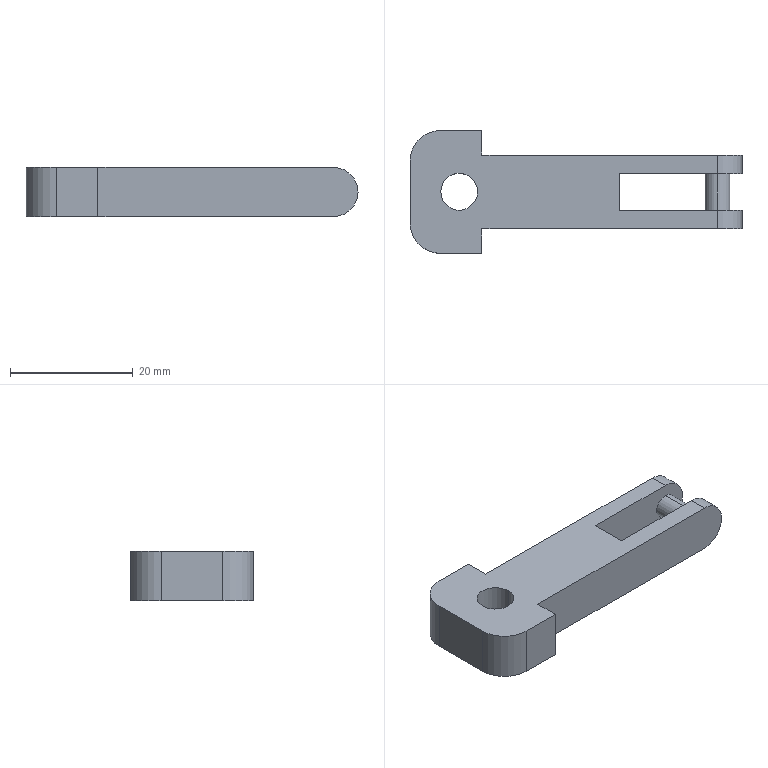Part | SolidWorks | features Fillet 2, ICE 2, Extrusion 1 | 1 solid | 22 faces | box 54 x 20 x 8 mm | volume 4696 mm3 | plane 12 | cylinder 10 | commonest cylinder face diameters 8 x4 4 x2 6 x2 10 x2
STEP:
#1=CARTESIAN_POINT('',(-27.268,0.,0.));
#2=VERTEX_POINT('',#1);
#3=CARTESIAN_POINT('',(-21.268,0.,0.));
#4=VERTEX_POINT('',#3);
#5=CARTESIAN_POINT('',(-24.268,0.,0.));
#6=DIRECTION('',(0.,0.,1.));
#7=DIRECTION('',(1.,0.,0.));
#8=AXIS2_PLACEMENT_3D('',#5,#6,#7);
#9=CIRCLE('',#8,3.);
#10=EDGE_CURVE('',#2,#4,#9,.T.);
#11=ORIENTED_EDGE('',*,*,#10,.F.);
#12=CARTESIAN_POINT('',(-27.268,0.,8.));
#13=VERTEX_POINT('',#12);
#14=CARTESIAN_POINT('',(-27.268,0.,0.));
#15=DIRECTION('',(0.,0.,1.));
#16=VECTOR('',#15,1000.);
#17=LINE('',#14,#16);
#18=EDGE_CURVE('',#2,#13,#17,.T.);
#19=ORIENTED_EDGE('',*,*,#18,.T.);
#20=CARTESIAN_POINT('',(-21.268,0.,8.));
#21=VERTEX_POINT('',#20);
#22=CARTESIAN_POINT('',(-24.268,0.,8.));
#23=DIRECTION('',(0.,0.,1.));
#24=DIRECTION('',(1.,0.,0.));
#25=AXIS2_PLACEMENT_3D('',#22,#23,#24);
#26=CIRCLE('',#25,3.);
#27=EDGE_CURVE('',#13,#21,#26,.T.);
#28=ORIENTED_EDGE('',*,*,#27,.T.);
#29=CARTESIAN_POINT('',(-21.268,0.,0.));
#30=DIRECTION('',(0.,0.,1.));
#31=VECTOR('',#30,1000.);
#32=LINE('',#29,#31);
#33=EDGE_CURVE('',#4,#21,#32,.T.);
#34=ORIENTED_EDGE('',*,*,#33,.F.);
#35=EDGE_LOOP('',(#11,#19,#28,#34));
#36=FACE_OUTER_BOUND('',#35,.T.);
#37=CARTESIAN_POINT('',(-24.268,0.,0.));
#38=DIRECTION('',(0.,0.,1.));
#39=DIRECTION('',(1.,0.,0.));
#40=AXIS2_PLACEMENT_3D('',#37,#38,#39);
#41=CYLINDRICAL_SURFACE('',#40,3.);
#42=ADVANCED_FACE('',(#36),#41,.F.);
#43=CARTESIAN_POINT('',(17.732,2.96,6.));
#44=VERTEX_POINT('',#43);
#45=CARTESIAN_POINT('',(17.732,2.96,2.));
#46=VERTEX_POINT('',#45);
#47=CARTESIAN_POINT('',(17.732,2.96,4.));
#48=DIRECTION('',(0.,1.,0.));
#49=DIRECTION('',(-1.,0.,0.));
#50=AXIS2_PLACEMENT_3D('',#47,#48,#49);
#51=CIRCLE('',#50,2.);
#52=EDGE_CURVE('',#44,#46,#51,.T.);
#53=ORIENTED_EDGE('',*,*,#52,.F.);
#54=CARTESIAN_POINT('',(17.732,-3.04,6.));
#55=VERTEX_POINT('',#54);
#56=CARTESIAN_POINT('',(17.732,5.96,6.));
#57=DIRECTION('',(0.,-1.,0.));
#58=VECTOR('',#57,1000.);
#59=LINE('',#56,#58);
#60=EDGE_CURVE('',#44,#55,#59,.T.);
#61=ORIENTED_EDGE('',*,*,#60,.T.);
#62=CARTESIAN_POINT('',(17.732,-3.04,2.));
#63=VERTEX_POINT('',#62);
#64=CARTESIAN_POINT('',(17.732,-3.04,4.));
#65=DIRECTION('',(0.,-1.,0.));
#66=DIRECTION('',(0.,0.,-1.));
#67=AXIS2_PLACEMENT_3D('',#64,#65,#66);
#68=CIRCLE('',#67,2.);
#69=EDGE_CURVE('',#63,#55,#68,.T.);
#70=ORIENTED_EDGE('',*,*,#69,.F.);
#71=CARTESIAN_POINT('',(17.732,5.96,2.));
#72=DIRECTION('',(0.,-1.,0.));
#73=VECTOR('',#72,1000.);
#74=LINE('',#71,#73);
#75=EDGE_CURVE('',#46,#63,#74,.T.);
#76=ORIENTED_EDGE('',*,*,#75,.F.);
#77=EDGE_LOOP('',(#53,#61,#70,#76));
#78=FACE_OUTER_BOUND('',#77,.T.);
#79=CARTESIAN_POINT('',(17.732,5.96,4.));
#80=DIRECTION('',(0.,-1.,0.));
#81=DIRECTION('',(0.,0.,-1.));
#82=AXIS2_PLACEMENT_3D('',#79,#80,#81);
#83=CYLINDRICAL_SURFACE('',#82,2.);
#84=ADVANCED_FACE('',(#78),#83,.T.);
#85=CARTESIAN_POINT('',(17.732,5.96,8.));
#86=VERTEX_POINT('',#85);
#87=CARTESIAN_POINT('',(21.732,5.96,4.));
#88=VERTEX_POINT('',#87);
#89=CARTESIAN_POINT('',(17.732,5.96,4.));
#90=DIRECTION('',(0.,1.,0.));
#91=DIRECTION('',(0.,0.,-1.));
#92=AXIS2_PLACEMENT_3D('',#89,#90,#91);
#93=CIRCLE('',#92,4.);
#94=EDGE_CURVE('',#86,#88,#93,.T.);
#95=ORIENTED_EDGE('',*,*,#94,.T.);
#96=CARTESIAN_POINT('',(17.732,5.96,0.));
#97=VERTEX_POINT('',#96);
#98=CARTESIAN_POINT('',(17.732,5.96,4.));
#99=DIRECTION('',(0.,1.,0.));
#100=DIRECTION('',(0.,0.,-1.));
#101=AXIS2_PLACEMENT_3D('',#98,#99,#100);
#102=CIRCLE('',#101,4.);
#103=EDGE_CURVE('',#88,#97,#102,.T.);
#104=ORIENTED_EDGE('',*,*,#103,.T.);
#105=CARTESIAN_POINT('',(-20.559,5.96,0.));
#106=VERTEX_POINT('',#105);
#107=CARTESIAN_POINT('',(-20.559,5.96,0.));
#108=DIRECTION('',(-1.,0.,0.));
#109=VECTOR('',#108,1000.);
#110=LINE('',#107,#109);
#111=EDGE_CURVE('',#97,#106,#110,.T.);
#112=ORIENTED_EDGE('',*,*,#111,.T.);
#113=CARTESIAN_POINT('',(-20.559,5.96,8.));
#114=VERTEX_POINT('',#113);
#115=CARTESIAN_POINT('',(-20.559,5.96,8.));
#116=DIRECTION('',(0.,0.,-1.));
#117=VECTOR('',#116,1000.);
#118=LINE('',#115,#117);
#119=EDGE_CURVE('',#114,#106,#118,.T.);
#120=ORIENTED_EDGE('',*,*,#119,.F.);
#121=CARTESIAN_POINT('',(-20.559,5.96,8.));
#122=DIRECTION('',(-1.,0.,0.));
#123=VECTOR('',#122,1000.);
#124=LINE('',#121,#123);
#125=EDGE_CURVE('',#86,#114,#124,.T.);
#126=ORIENTED_EDGE('',*,*,#125,.F.);
#127=EDGE_LOOP('',(#95,#104,#112,#120,#126));
#128=FACE_OUTER_BOUND('',#127,.T.);
#129=CARTESIAN_POINT('',(-20.559,5.96,8.));
#130=DIRECTION('',(0.,-1.,0.));
#131=DIRECTION('',(0.,0.,-1.));
#132=AXIS2_PLACEMENT_3D('',#129,#130,#131);
#133=PLANE('',#132);
#134=ADVANCED_FACE('',(#128),#133,.F.);
#135=CARTESIAN_POINT('',(-20.559,9.96,0.));
#136=VERTEX_POINT('',#135);
#137=CARTESIAN_POINT('',(-20.559,9.96,0.));
#138=DIRECTION('',(0.,1.,0.));
#139=VECTOR('',#138,1000.);
#140=LINE('',#137,#139);
#141=EDGE_CURVE('',#106,#136,#140,.T.);
#142=ORIENTED_EDGE('',*,*,#141,.T.);
#143=CARTESIAN_POINT('',(-20.559,9.96,8.));
#144=VERTEX_POINT('',#143);
#145=CARTESIAN_POINT('',(-20.559,9.96,8.));
#146=DIRECTION('',(0.,0.,-1.));
#147=VECTOR('',#146,1000.);
#148=LINE('',#145,#147);
#149=EDGE_CURVE('',#144,#136,#148,.T.);
#150=ORIENTED_EDGE('',*,*,#149,.F.);
#151=CARTESIAN_POINT('',(-20.559,9.96,8.));
#152=DIRECTION('',(0.,1.,0.));
#153=VECTOR('',#152,1000.);
#154=LINE('',#151,#153);
#155=EDGE_CURVE('',#114,#144,#154,.T.);
#156=ORIENTED_EDGE('',*,*,#155,.F.);
#157=ORIENTED_EDGE('',*,*,#119,.T.);
#158=EDGE_LOOP('',(#142,#150,#156,#157));
#159=FACE_OUTER_BOUND('',#158,.T.);
#160=CARTESIAN_POINT('',(-20.559,9.96,8.));
#161=DIRECTION('',(-1.,0.,0.));
#162=DIRECTION('',(0.,0.,1.));
#163=AXIS2_PLACEMENT_3D('',#160,#161,#162);
#164=PLANE('',#163);
#165=ADVANCED_FACE('',(#159),#164,.F.);
#166=CARTESIAN_POINT('',(-27.268,9.96,0.));
#167=VERTEX_POINT('',#166);
#168=CARTESIAN_POINT('',(-20.559,9.96,0.));
#169=DIRECTION('',(-1.,0.,0.));
#170=VECTOR('',#169,1000.);
#171=LINE('',#168,#170);
#172=EDGE_CURVE('',#136,#167,#171,.T.);
#173=ORIENTED_EDGE('',*,*,#172,.T.);
#174=CARTESIAN_POINT('',(-27.268,9.96,8.));
#175=VERTEX_POINT('',#174);
#176=CARTESIAN_POINT('',(-27.268,9.96,8.));
#177=DIRECTION('',(0.,0.,1.));
#178=VECTOR('',#177,1000.);
#179=LINE('',#176,#178);
#180=EDGE_CURVE('',#167,#175,#179,.T.);
#181=ORIENTED_EDGE('',*,*,#180,.T.);
#182=CARTESIAN_POINT('',(-20.559,9.96,8.));
#183=DIRECTION('',(-1.,0.,0.));
#184=VECTOR('',#183,1000.);
#185=LINE('',#182,#184);
#186=EDGE_CURVE('',#144,#175,#185,.T.);
#187=ORIENTED_EDGE('',*,*,#186,.F.);
#188=ORIENTED_EDGE('',*,*,#149,.T.);
#189=EDGE_LOOP('',(#173,#181,#187,#188));
#190=FACE_OUTER_BOUND('',#189,.T.);
#191=CARTESIAN_POINT('',(-20.559,9.96,8.));
#192=DIRECTION('',(0.,-1.,0.));
#193=DIRECTION('',(0.,0.,-1.));
#194=AXIS2_PLACEMENT_3D('',#191,#192,#193);
#195=PLANE('',#194);
#196=ADVANCED_FACE('',(#190),#195,.F.);
#197=CARTESIAN_POINT('',(-32.268,4.96,0.));
#198=VERTEX_POINT('',#197);
#199=CARTESIAN_POINT('',(-32.268,-5.04,0.));
#200=VERTEX_POINT('',#199);
#201=CARTESIAN_POINT('',(-32.268,-10.04,0.));
#202=DIRECTION('',(0.,-1.,0.));
#203=VECTOR('',#202,1000.);
#204=LINE('',#201,#203);
#205=EDGE_CURVE('',#198,#200,#204,.T.);
#206=ORIENTED_EDGE('',*,*,#205,.T.);
#207=CARTESIAN_POINT('',(-32.268,-5.04,8.));
#208=VERTEX_POINT('',#207);
#209=CARTESIAN_POINT('',(-32.268,-5.04,8.));
#210=DIRECTION('',(0.,0.,1.));
#211=VECTOR('',#210,1000.);
#212=LINE('',#209,#211);
#213=EDGE_CURVE('',#200,#208,#212,.T.);
#214=ORIENTED_EDGE('',*,*,#213,.T.);
#215=CARTESIAN_POINT('',(-32.268,4.96,8.));
#216=VERTEX_POINT('',#215);
#217=CARTESIAN_POINT('',(-32.268,9.96,8.));
#218=DIRECTION('',(0.,-1.,0.));
#219=VECTOR('',#218,1000.);
#220=LINE('',#217,#219);
#221=EDGE_CURVE('',#216,#208,#220,.T.);
#222=ORIENTED_EDGE('',*,*,#221,.F.);
#223=CARTESIAN_POINT('',(-32.268,4.96,8.));
#224=DIRECTION('',(0.,0.,-1.));
#225=VECTOR('',#224,1000.);
#226=LINE('',#223,#225);
#227=EDGE_CURVE('',#216,#198,#226,.T.);
#228=ORIENTED_EDGE('',*,*,#227,.T.);
#229=EDGE_LOOP('',(#206,#214,#222,#228));
#230=FACE_OUTER_BOUND('',#229,.T.);
#231=CARTESIAN_POINT('',(-32.268,-10.04,8.));
#232=DIRECTION('',(1.,0.,0.));
#233=DIRECTION('',(0.,0.,-1.));
#234=AXIS2_PLACEMENT_3D('',#231,#232,#233);
#235=PLANE('',#234);
#236=ADVANCED_FACE('',(#230),#235,.F.);
#237=CARTESIAN_POINT('',(-27.268,-10.04,8.));
#238=VERTEX_POINT('',#237);
#239=CARTESIAN_POINT('',(-20.559,-10.04,8.));
#240=VERTEX_POINT('',#239);
#241=CARTESIAN_POINT('',(-32.268,-10.04,8.));
#242=DIRECTION('',(1.,0.,0.));
#243=VECTOR('',#242,1000.);
#244=LINE('',#241,#243);
#245=EDGE_CURVE('',#238,#240,#244,.T.);
#246=ORIENTED_EDGE('',*,*,#245,.F.);
#247=CARTESIAN_POINT('',(-27.268,-10.04,0.));
#248=VERTEX_POINT('',#247);
#249=CARTESIAN_POINT('',(-27.268,-10.04,8.));
#250=DIRECTION('',(0.,0.,-1.));
#251=VECTOR('',#250,1000.);
#252=LINE('',#249,#251);
#253=EDGE_CURVE('',#238,#248,#252,.T.);
#254=ORIENTED_EDGE('',*,*,#253,.T.);
#255=CARTESIAN_POINT('',(-20.559,-10.04,0.));
#256=VERTEX_POINT('',#255);
#257=CARTESIAN_POINT('',(-32.268,-10.04,0.));
#258=DIRECTION('',(1.,0.,0.));
#259=VECTOR('',#258,1000.);
#260=LINE('',#257,#259);
#261=EDGE_CURVE('',#248,#256,#260,.T.);
#262=ORIENTED_EDGE('',*,*,#261,.T.);
#263=CARTESIAN_POINT('',(-20.559,-10.04,8.));
#264=DIRECTION('',(0.,0.,-1.));
#265=VECTOR('',#264,1000.);
#266=LINE('',#263,#265);
#267=EDGE_CURVE('',#240,#256,#266,.T.);
#268=ORIENTED_EDGE('',*,*,#267,.F.);
#269=EDGE_LOOP('',(#246,#254,#262,#268));
#270=FACE_OUTER_BOUND('',#269,.T.);
#271=CARTESIAN_POINT('',(-32.268,-10.04,8.));
#272=DIRECTION('',(0.,1.,0.));
#273=DIRECTION('',(0.,0.,1.));
#274=AXIS2_PLACEMENT_3D('',#271,#272,#273);
#275=PLANE('',#274);
#276=ADVANCED_FACE('',(#270),#275,.F.);
#277=CARTESIAN_POINT('',(-20.559,-6.04,0.));
#278=VERTEX_POINT('',#277);
#279=CARTESIAN_POINT('',(-20.559,-6.04,0.));
#280=DIRECTION('',(0.,1.,0.));
#281=VECTOR('',#280,1000.);
#282=LINE('',#279,#281);
#283=EDGE_CURVE('',#256,#278,#282,.T.);
#284=ORIENTED_EDGE('',*,*,#283,.T.);
#285=CARTESIAN_POINT('',(-20.559,-6.04,8.));
#286=VERTEX_POINT('',#285);
#287=CARTESIAN_POINT('',(-20.559,-6.04,8.));
#288=DIRECTION('',(0.,0.,-1.));
#289=VECTOR('',#288,1000.);
#290=LINE('',#287,#289);
#291=EDGE_CURVE('',#286,#278,#290,.T.);
#292=ORIENTED_EDGE('',*,*,#291,.F.);
#293=CARTESIAN_POINT('',(-20.559,-6.04,8.));
#294=DIRECTION('',(0.,1.,0.));
#295=VECTOR('',#294,1000.);
#296=LINE('',#293,#295);
#297=EDGE_CURVE('',#240,#286,#296,.T.);
#298=ORIENTED_EDGE('',*,*,#297,.F.);
#299=ORIENTED_EDGE('',*,*,#267,.T.);
#300=EDGE_LOOP('',(#284,#292,#298,#299));
#301=FACE_OUTER_BOUND('',#300,.T.);
#302=CARTESIAN_POINT('',(-20.559,-6.04,8.));
#303=DIRECTION('',(-1.,0.,0.));
#304=DIRECTION('',(0.,0.,1.));
#305=AXIS2_PLACEMENT_3D('',#302,#303,#304);
#306=PLANE('',#305);
#307=ADVANCED_FACE('',(#301),#306,.F.);
#308=CARTESIAN_POINT('',(17.732,-6.04,0.));
#309=VERTEX_POINT('',#308);
#310=CARTESIAN_POINT('',(-20.559,-6.04,0.));
#311=DIRECTION('',(1.,0.,0.));
#312=VECTOR('',#311,1000.);
#313=LINE('',#310,#312);
#314=EDGE_CURVE('',#278,#309,#313,.T.);
#315=ORIENTED_EDGE('',*,*,#314,.T.);
#316=CARTESIAN_POINT('',(21.732,-6.04,4.));
#317=VERTEX_POINT('',#316);
#318=CARTESIAN_POINT('',(17.732,-6.04,4.));
#319=DIRECTION('',(0.,-1.,0.));
#320=DIRECTION('',(0.,0.,1.));
#321=AXIS2_PLACEMENT_3D('',#318,#319,#320);
#322=CIRCLE('',#321,4.);
#323=EDGE_CURVE('',#309,#317,#322,.T.);
#324=ORIENTED_EDGE('',*,*,#323,.T.);
#325=CARTESIAN_POINT('',(17.732,-6.04,8.));
#326=VERTEX_POINT('',#325);
#327=CARTESIAN_POINT('',(17.732,-6.04,4.));
#328=DIRECTION('',(0.,-1.,0.));
#329=DIRECTION('',(0.,0.,1.));
#330=AXIS2_PLACEMENT_3D('',#327,#328,#329);
#331=CIRCLE('',#330,4.);
#332=EDGE_CURVE('',#317,#326,#331,.T.);
#333=ORIENTED_EDGE('',*,*,#332,.T.);
#334=CARTESIAN_POINT('',(-20.559,-6.04,8.));
#335=DIRECTION('',(1.,0.,0.));
#336=VECTOR('',#335,1000.);
#337=LINE('',#334,#336);
#338=EDGE_CURVE('',#286,#326,#337,.T.);
#339=ORIENTED_EDGE('',*,*,#338,.F.);
#340=ORIENTED_EDGE('',*,*,#291,.T.);
#341=EDGE_LOOP('',(#315,#324,#333,#339,#340));
#342=FACE_OUTER_BOUND('',#341,.T.);
#343=CARTESIAN_POINT('',(-20.559,-6.04,8.));
#344=DIRECTION('',(0.,1.,0.));
#345=DIRECTION('',(0.,0.,1.));
#346=AXIS2_PLACEMENT_3D('',#343,#344,#345);
#347=PLANE('',#346);
#348=ADVANCED_FACE('',(#342),#347,.F.);
#349=ORIENTED_EDGE('',*,*,#69,.T.);
#350=CARTESIAN_POINT('',(17.732,-3.04,4.));
#351=DIRECTION('',(0.,-1.,0.));
#352=DIRECTION('',(0.,0.,-1.));
#353=AXIS2_PLACEMENT_3D('',#350,#351,#352);
#354=CIRCLE('',#353,2.);
#355=EDGE_CURVE('',#55,#63,#354,.T.);
#356=ORIENTED_EDGE('',*,*,#355,.T.);
#357=EDGE_LOOP('',(#349,#356));
#358=FACE_BOUND('',#357,.T.);
#359=CARTESIAN_POINT('',(17.732,-3.04,8.));
#360=VERTEX_POINT('',#359);
#361=CARTESIAN_POINT('',(21.732,-3.04,4.));
#362=VERTEX_POINT('',#361);
#363=CARTESIAN_POINT('',(17.732,-3.04,4.));
#364=DIRECTION('',(0.,1.,0.));
#365=DIRECTION('',(0.,0.,-1.));
#366=AXIS2_PLACEMENT_3D('',#363,#364,#365);
#367=CIRCLE('',#366,4.);
#368=EDGE_CURVE('',#360,#362,#367,.T.);
#369=ORIENTED_EDGE('',*,*,#368,.T.);
#370=CARTESIAN_POINT('',(17.732,-3.04,0.));
#371=VERTEX_POINT('',#370);
#372=CARTESIAN_POINT('',(17.732,-3.04,4.));
#373=DIRECTION('',(0.,1.,0.));
#374=DIRECTION('',(0.,0.,-1.));
#375=AXIS2_PLACEMENT_3D('',#372,#373,#374);
#376=CIRCLE('',#375,4.);
#377=EDGE_CURVE('',#362,#371,#376,.T.);
#378=ORIENTED_EDGE('',*,*,#377,.T.);
#379=CARTESIAN_POINT('',(1.732,-3.04,0.));
#380=VERTEX_POINT('',#379);
#381=CARTESIAN_POINT('',(1.732,-3.04,0.));
#382=DIRECTION('',(-1.,0.,0.));
#383=VECTOR('',#382,1000.);
#384=LINE('',#381,#383);
#385=EDGE_CURVE('',#371,#380,#384,.T.);
#386=ORIENTED_EDGE('',*,*,#385,.T.);
#387=CARTESIAN_POINT('',(1.732,-3.04,8.));
#388=VERTEX_POINT('',#387);
#389=CARTESIAN_POINT('',(1.732,-3.04,8.));
#390=DIRECTION('',(0.,0.,-1.));
#391=VECTOR('',#390,1000.);
#392=LINE('',#389,#391);
#393=EDGE_CURVE('',#388,#380,#392,.T.);
#394=ORIENTED_EDGE('',*,*,#393,.F.);
#395=CARTESIAN_POINT('',(1.732,-3.04,8.));
#396=DIRECTION('',(-1.,0.,0.));
#397=VECTOR('',#396,1000.);
#398=LINE('',#395,#397);
#399=EDGE_CURVE('',#360,#388,#398,.T.);
#400=ORIENTED_EDGE('',*,*,#399,.F.);
#401=EDGE_LOOP('',(#369,#378,#386,#394,#400));
#402=FACE_OUTER_BOUND('',#401,.T.);
#403=CARTESIAN_POINT('',(1.732,-3.04,8.));
#404=DIRECTION('',(0.,-1.,0.));
#405=DIRECTION('',(0.,0.,-1.));
#406=AXIS2_PLACEMENT_3D('',#403,#404,#405);
#407=PLANE('',#406);
#408=ADVANCED_FACE('',(#358,#402),#407,.F.);
#409=CARTESIAN_POINT('',(1.732,2.96,0.));
#410=VERTEX_POINT('',#409);
#411=CARTESIAN_POINT('',(1.732,2.96,0.));
#412=DIRECTION('',(0.,1.,0.));
#413=VECTOR('',#412,1000.);
#414=LINE('',#411,#413);
#415=EDGE_CURVE('',#380,#410,#414,.T.);
#416=ORIENTED_EDGE('',*,*,#415,.T.);
#417=CARTESIAN_POINT('',(1.732,2.96,8.));
#418=VERTEX_POINT('',#417);
#419=CARTESIAN_POINT('',(1.732,2.96,8.));
#420=DIRECTION('',(0.,0.,-1.));
#421=VECTOR('',#420,1000.);
#422=LINE('',#419,#421);
#423=EDGE_CURVE('',#418,#410,#422,.T.);
#424=ORIENTED_EDGE('',*,*,#423,.F.);
#425=CARTESIAN_POINT('',(1.732,2.96,8.));
#426=DIRECTION('',(0.,1.,0.));
#427=VECTOR('',#426,1000.);
#428=LINE('',#425,#427);
#429=EDGE_CURVE('',#388,#418,#428,.T.);
#430=ORIENTED_EDGE('',*,*,#429,.F.);
#431=ORIENTED_EDGE('',*,*,#393,.T.);
#432=EDGE_LOOP('',(#416,#424,#430,#431));
#433=FACE_OUTER_BOUND('',#432,.T.);
#434=CARTESIAN_POINT('',(1.732,2.96,8.));
#435=DIRECTION('',(-1.,0.,0.));
#436=DIRECTION('',(0.,0.,1.));
#437=AXIS2_PLACEMENT_3D('',#434,#435,#436);
#438=PLANE('',#437);
#439=ADVANCED_FACE('',(#433),#438,.F.);
#440=CARTESIAN_POINT('',(17.732,2.96,4.));
#441=DIRECTION('',(0.,1.,0.));
#442=DIRECTION('',(-1.,0.,0.));
#443=AXIS2_PLACEMENT_3D('',#440,#441,#442);
#444=CIRCLE('',#443,2.);
#445=EDGE_CURVE('',#46,#44,#444,.T.);
#446=ORIENTED_EDGE('',*,*,#445,.T.);
#447=ORIENTED_EDGE('',*,*,#52,.T.);
#448=EDGE_LOOP('',(#446,#447));
#449=FACE_BOUND('',#448,.T.);
#450=CARTESIAN_POINT('',(17.732,2.96,0.));
#451=VERTEX_POINT('',#450);
#452=CARTESIAN_POINT('',(1.732,2.96,0.));
#453=DIRECTION('',(1.,0.,0.));
#454=VECTOR('',#453,1000.);
#455=LINE('',#452,#454);
#456=EDGE_CURVE('',#410,#451,#455,.T.);
#457=ORIENTED_EDGE('',*,*,#456,.T.);
#458=CARTESIAN_POINT('',(21.732,2.96,4.));
#459=VERTEX_POINT('',#458);
#460=CARTESIAN_POINT('',(17.732,2.96,4.));
#461=DIRECTION('',(0.,-1.,0.));
#462=DIRECTION('',(-1.,0.,0.));
#463=AXIS2_PLACEMENT_3D('',#460,#461,#462);
#464=CIRCLE('',#463,4.);
#465=EDGE_CURVE('',#451,#459,#464,.T.);
#466=ORIENTED_EDGE('',*,*,#465,.T.);
#467=CARTESIAN_POINT('',(17.732,2.96,8.));
#468=VERTEX_POINT('',#467);
#469=CARTESIAN_POINT('',(17.732,2.96,4.));
#470=DIRECTION('',(0.,-1.,0.));
#471=DIRECTION('',(-1.,0.,0.));
#472=AXIS2_PLACEMENT_3D('',#469,#470,#471);
#473=CIRCLE('',#472,4.);
#474=EDGE_CURVE('',#459,#468,#473,.T.);
#475=ORIENTED_EDGE('',*,*,#474,.T.);
#476=CARTESIAN_POINT('',(1.732,2.96,8.));
#477=DIRECTION('',(1.,0.,0.));
#478=VECTOR('',#477,1000.);
#479=LINE('',#476,#478);
#480=EDGE_CURVE('',#418,#468,#479,.T.);
#481=ORIENTED_EDGE('',*,*,#480,.F.);
#482=ORIENTED_EDGE('',*,*,#423,.T.);
#483=EDGE_LOOP('',(#457,#466,#475,#481,#482));
#484=FACE_OUTER_BOUND('',#483,.T.);
#485=CARTESIAN_POINT('',(1.732,2.96,8.));
#486=DIRECTION('',(0.,1.,0.));
#487=DIRECTION('',(-1.,0.,0.));
#488=AXIS2_PLACEMENT_3D('',#485,#486,#487);
#489=PLANE('',#488);
#490=ADVANCED_FACE('',(#449,#484),#489,.F.);
#491=CARTESIAN_POINT('',(-24.268,0.,8.));
#492=DIRECTION('',(0.,0.,1.));
#493=DIRECTION('',(1.,0.,0.));
#494=AXIS2_PLACEMENT_3D('',#491,#492,#493);
#495=CIRCLE('',#494,3.);
#496=EDGE_CURVE('',#21,#13,#495,.T.);
#497=ORIENTED_EDGE('',*,*,#496,.F.);
#498=ORIENTED_EDGE('',*,*,#27,.F.);
#499=EDGE_LOOP('',(#497,#498));
#500=FACE_BOUND('',#499,.T.);
#501=ORIENTED_EDGE('',*,*,#338,.T.);
#502=CARTESIAN_POINT('',(17.732,0.,8.));
#503=DIRECTION('',(0.,1.,0.));
#504=VECTOR('',#503,1000.);
#505=LINE('',#502,#504);
#506=EDGE_CURVE('',#326,#360,#505,.T.);
#507=ORIENTED_EDGE('',*,*,#506,.T.);
#508=ORIENTED_EDGE('',*,*,#399,.T.);
#509=ORIENTED_EDGE('',*,*,#429,.T.);
#510=ORIENTED_EDGE('',*,*,#480,.T.);
#511=CARTESIAN_POINT('',(17.732,0.,8.));
#512=DIRECTION('',(0.,1.,0.));
#513=VECTOR('',#512,1000.);
#514=LINE('',#511,#513);
#515=EDGE_CURVE('',#468,#86,#514,.T.);
#516=ORIENTED_EDGE('',*,*,#515,.T.);
#517=ORIENTED_EDGE('',*,*,#125,.T.);
#518=ORIENTED_EDGE('',*,*,#155,.T.);
#519=ORIENTED_EDGE('',*,*,#186,.T.);
#520=CARTESIAN_POINT('',(-27.268,4.96,8.));
#521=DIRECTION('',(0.,0.,1.));
#522=DIRECTION('',(-1.,0.,0.));
#523=AXIS2_PLACEMENT_3D('',#520,#521,#522);
#524=CIRCLE('',#523,5.);
#525=EDGE_CURVE('',#175,#216,#524,.T.);
#526=ORIENTED_EDGE('',*,*,#525,.T.);
#527=ORIENTED_EDGE('',*,*,#221,.T.);
#528=CARTESIAN_POINT('',(-27.268,-5.04,8.));
#529=DIRECTION('',(0.,0.,1.));
#530=DIRECTION('',(-1.,0.,0.));
#531=AXIS2_PLACEMENT_3D('',#528,#529,#530);
#532=CIRCLE('',#531,5.);
#533=EDGE_CURVE('',#208,#238,#532,.T.);
#534=ORIENTED_EDGE('',*,*,#533,.T.);
#535=ORIENTED_EDGE('',*,*,#245,.T.);
#536=ORIENTED_EDGE('',*,*,#297,.T.);
#537=EDGE_LOOP('',(#501,#507,#508,#509,#510,#516,#517,#518,#519,#526,#527,#534,#535,#536));
#538=FACE_OUTER_BOUND('',#537,.T.);
#539=CARTESIAN_POINT('',(0.,0.,8.));
#540=DIRECTION('',(0.,0.,-1.));
#541=DIRECTION('',(-1.,0.,0.));
#542=AXIS2_PLACEMENT_3D('',#539,#540,#541);
#543=PLANE('',#542);
#544=ADVANCED_FACE('',(#500,#538),#543,.F.);
#545=CARTESIAN_POINT('',(-24.268,0.,0.));
#546=DIRECTION('',(0.,0.,1.));
#547=DIRECTION('',(1.,0.,0.));
#548=AXIS2_PLACEMENT_3D('',#545,#546,#547);
#549=CIRCLE('',#548,3.);
#550=EDGE_CURVE('',#4,#2,#549,.T.);
#551=ORIENTED_EDGE('',*,*,#550,.T.);
#552=ORIENTED_EDGE('',*,*,#10,.T.);
#553=EDGE_LOOP('',(#551,#552));
#554=FACE_BOUND('',#553,.T.);
#555=ORIENTED_EDGE('',*,*,#385,.F.);
#556=CARTESIAN_POINT('',(17.732,-6.04,0.));
#557=DIRECTION('',(0.,-1.,0.));
#558=VECTOR('',#557,1000.);
#559=LINE('',#556,#558);
#560=EDGE_CURVE('',#371,#309,#559,.T.);
#561=ORIENTED_EDGE('',*,*,#560,.T.);
#562=ORIENTED_EDGE('',*,*,#314,.F.);
#563=ORIENTED_EDGE('',*,*,#283,.F.);
#564=ORIENTED_EDGE('',*,*,#261,.F.);
#565=CARTESIAN_POINT('',(-27.268,-5.04,0.));
#566=DIRECTION('',(0.,0.,-1.));
#567=DIRECTION('',(-1.,0.,0.));
#568=AXIS2_PLACEMENT_3D('',#565,#566,#567);
#569=CIRCLE('',#568,5.);
#570=EDGE_CURVE('',#248,#200,#569,.T.);
#571=ORIENTED_EDGE('',*,*,#570,.T.);
#572=ORIENTED_EDGE('',*,*,#205,.F.);
#573=CARTESIAN_POINT('',(-27.268,4.96,0.));
#574=DIRECTION('',(0.,0.,-1.));
#575=DIRECTION('',(-1.,0.,0.));
#576=AXIS2_PLACEMENT_3D('',#573,#574,#575);
#577=CIRCLE('',#576,5.);
#578=EDGE_CURVE('',#198,#167,#577,.T.);
#579=ORIENTED_EDGE('',*,*,#578,.T.);
#580=ORIENTED_EDGE('',*,*,#172,.F.);
#581=ORIENTED_EDGE('',*,*,#141,.F.);
#582=ORIENTED_EDGE('',*,*,#111,.F.);
#583=CARTESIAN_POINT('',(17.732,2.96,0.));
#584=DIRECTION('',(0.,-1.,0.));
#585=VECTOR('',#584,1000.);
#586=LINE('',#583,#585);
#587=EDGE_CURVE('',#97,#451,#586,.T.);
#588=ORIENTED_EDGE('',*,*,#587,.T.);
#589=ORIENTED_EDGE('',*,*,#456,.F.);
#590=ORIENTED_EDGE('',*,*,#415,.F.);
#591=EDGE_LOOP('',(#555,#561,#562,#563,#564,#571,#572,#579,#580,#581,#582,#588,#589,#590));
#592=FACE_OUTER_BOUND('',#591,.T.);
#593=CARTESIAN_POINT('',(0.,0.,0.));
#594=DIRECTION('',(0.,0.,-1.));
#595=DIRECTION('',(-1.,0.,0.));
#596=AXIS2_PLACEMENT_3D('',#593,#594,#595);
#597=PLANE('',#596);
#598=ADVANCED_FACE('',(#554,#592),#597,.T.);
#599=ORIENTED_EDGE('',*,*,#533,.F.);
#600=ORIENTED_EDGE('',*,*,#213,.F.);
#601=ORIENTED_EDGE('',*,*,#570,.F.);
#602=ORIENTED_EDGE('',*,*,#253,.F.);
#603=EDGE_LOOP('',(#599,#600,#601,#602));
#604=FACE_OUTER_BOUND('',#603,.T.);
#605=CARTESIAN_POINT('',(-27.268,-5.04,8.));
#606=DIRECTION('',(0.,0.,-1.));
#607=DIRECTION('',(-1.,0.,0.));
#608=AXIS2_PLACEMENT_3D('',#605,#606,#607);
#609=CYLINDRICAL_SURFACE('',#608,5.);
#610=ADVANCED_FACE('',(#604),#609,.T.);
#611=ORIENTED_EDGE('',*,*,#525,.F.);
#612=ORIENTED_EDGE('',*,*,#180,.F.);
#613=ORIENTED_EDGE('',*,*,#578,.F.);
#614=ORIENTED_EDGE('',*,*,#227,.F.);
#615=EDGE_LOOP('',(#611,#612,#613,#614));
#616=FACE_OUTER_BOUND('',#615,.T.);
#617=CARTESIAN_POINT('',(-27.268,4.96,8.));
#618=DIRECTION('',(0.,0.,-1.));
#619=DIRECTION('',(-1.,0.,0.));
#620=AXIS2_PLACEMENT_3D('',#617,#618,#619);
#621=CYLINDRICAL_SURFACE('',#620,5.);
#622=ADVANCED_FACE('',(#616),#621,.T.);
#623=ORIENTED_EDGE('',*,*,#506,.F.);
#624=ORIENTED_EDGE('',*,*,#332,.F.);
#625=CARTESIAN_POINT('',(21.732,-6.04,4.));
#626=DIRECTION('',(0.,-1.,0.));
#627=VECTOR('',#626,1000.);
#628=LINE('',#625,#627);
#629=EDGE_CURVE('',#362,#317,#628,.T.);
#630=ORIENTED_EDGE('',*,*,#629,.F.);
#631=ORIENTED_EDGE('',*,*,#368,.F.);
#632=EDGE_LOOP('',(#623,#624,#630,#631));
#633=FACE_OUTER_BOUND('',#632,.T.);
#634=CARTESIAN_POINT('',(17.732,0.,4.));
#635=DIRECTION('',(0.,1.,0.));
#636=DIRECTION('',(0.,0.,1.));
#637=AXIS2_PLACEMENT_3D('',#634,#635,#636);
#638=CYLINDRICAL_SURFACE('',#637,4.);
#639=ADVANCED_FACE('',(#633),#638,.T.);
#640=ORIENTED_EDGE('',*,*,#323,.F.);
#641=ORIENTED_EDGE('',*,*,#560,.F.);
#642=ORIENTED_EDGE('',*,*,#377,.F.);
#643=ORIENTED_EDGE('',*,*,#629,.T.);
#644=EDGE_LOOP('',(#640,#641,#642,#643));
#645=FACE_OUTER_BOUND('',#644,.T.);
#646=CARTESIAN_POINT('',(17.732,-6.04,4.));
#647=DIRECTION('',(0.,-1.,0.));
#648=DIRECTION('',(0.,0.,-1.));
#649=AXIS2_PLACEMENT_3D('',#646,#647,#648);
#650=CYLINDRICAL_SURFACE('',#649,4.);
#651=ADVANCED_FACE('',(#645),#650,.T.);
#652=ORIENTED_EDGE('',*,*,#515,.F.);
#653=ORIENTED_EDGE('',*,*,#474,.F.);
#654=CARTESIAN_POINT('',(21.732,2.96,4.));
#655=DIRECTION('',(0.,-1.,0.));
#656=VECTOR('',#655,1000.);
#657=LINE('',#654,#656);
#658=EDGE_CURVE('',#88,#459,#657,.T.);
#659=ORIENTED_EDGE('',*,*,#658,.F.);
#660=ORIENTED_EDGE('',*,*,#94,.F.);
#661=EDGE_LOOP('',(#652,#653,#659,#660));
#662=FACE_OUTER_BOUND('',#661,.T.);
#663=CARTESIAN_POINT('',(17.732,0.,4.));
#664=DIRECTION('',(0.,1.,0.));
#665=DIRECTION('',(0.,0.,1.));
#666=AXIS2_PLACEMENT_3D('',#663,#664,#665);
#667=CYLINDRICAL_SURFACE('',#666,4.);
#668=ADVANCED_FACE('',(#662),#667,.T.);
#669=ORIENTED_EDGE('',*,*,#465,.F.);
#670=ORIENTED_EDGE('',*,*,#587,.F.);
#671=ORIENTED_EDGE('',*,*,#103,.F.);
#672=ORIENTED_EDGE('',*,*,#658,.T.);
#673=EDGE_LOOP('',(#669,#670,#671,#672));
#674=FACE_OUTER_BOUND('',#673,.T.);
#675=CARTESIAN_POINT('',(17.732,2.96,4.));
#676=DIRECTION('',(0.,-1.,0.));
#677=DIRECTION('',(0.,0.,-1.));
#678=AXIS2_PLACEMENT_3D('',#675,#676,#677);
#679=CYLINDRICAL_SURFACE('',#678,4.);
#680=ADVANCED_FACE('',(#674),#679,.T.);
#681=ORIENTED_EDGE('',*,*,#60,.F.);
#682=ORIENTED_EDGE('',*,*,#445,.F.);
#683=ORIENTED_EDGE('',*,*,#75,.T.);
#684=ORIENTED_EDGE('',*,*,#355,.F.);
#685=EDGE_LOOP('',(#681,#682,#683,#684));
#686=FACE_OUTER_BOUND('',#685,.T.);
#687=CARTESIAN_POINT('',(17.732,5.96,4.));
#688=DIRECTION('',(0.,-1.,0.));
#689=DIRECTION('',(0.,0.,-1.));
#690=AXIS2_PLACEMENT_3D('',#687,#688,#689);
#691=CYLINDRICAL_SURFACE('',#690,2.);
#692=ADVANCED_FACE('',(#686),#691,.T.);
#693=ORIENTED_EDGE('',*,*,#18,.F.);
#694=ORIENTED_EDGE('',*,*,#550,.F.);
#695=ORIENTED_EDGE('',*,*,#33,.T.);
#696=ORIENTED_EDGE('',*,*,#496,.T.);
#697=EDGE_LOOP('',(#693,#694,#695,#696));
#698=FACE_OUTER_BOUND('',#697,.T.);
#699=CARTESIAN_POINT('',(-24.268,0.,0.));
#700=DIRECTION('',(0.,0.,1.));
#701=DIRECTION('',(1.,0.,0.));
#702=AXIS2_PLACEMENT_3D('',#699,#700,#701);
#703=CYLINDRICAL_SURFACE('',#702,3.);
#704=ADVANCED_FACE('',(#698),#703,.F.);
#705=CLOSED_SHELL('',(#42,#84,#134,#165,#196,#236,#276,#307,#348,#408,#439,#490,#544,#598,#610,#622,#639,#651,#668,#680,#692,#704));
#706=MANIFOLD_SOLID_BREP('',#705);
#707=CARTESIAN_POINT('',(0.,0.,0.));
#708=DIRECTION('',(0.,0.,1.));
#709=DIRECTION('',(1.,0.,0.));
#710=AXIS2_PLACEMENT_3D('',#707,#708,#709);
#711=(LENGTH_UNIT()NAMED_UNIT(*)SI_UNIT(.MILLI.,.METRE.));
#712=UNCERTAINTY_MEASURE_WITH_UNIT(LENGTH_MEASURE(0.00001),#711,'','');
#713=(NAMED_UNIT(*)PLANE_ANGLE_UNIT()SI_UNIT($,.RADIAN.));
#714=(NAMED_UNIT(*)SI_UNIT($,.STERADIAN.)SOLID_ANGLE_UNIT());
#715=(GEOMETRIC_REPRESENTATION_CONTEXT(3)GLOBAL_UNCERTAINTY_ASSIGNED_CONTEXT((#712))GLOBAL_UNIT_ASSIGNED_CONTEXT((#711,#713,#714))REPRESENTATION_CONTEXT('',''));
#716=ADVANCED_BREP_SHAPE_REPRESENTATION('',(#706,#710),#715);